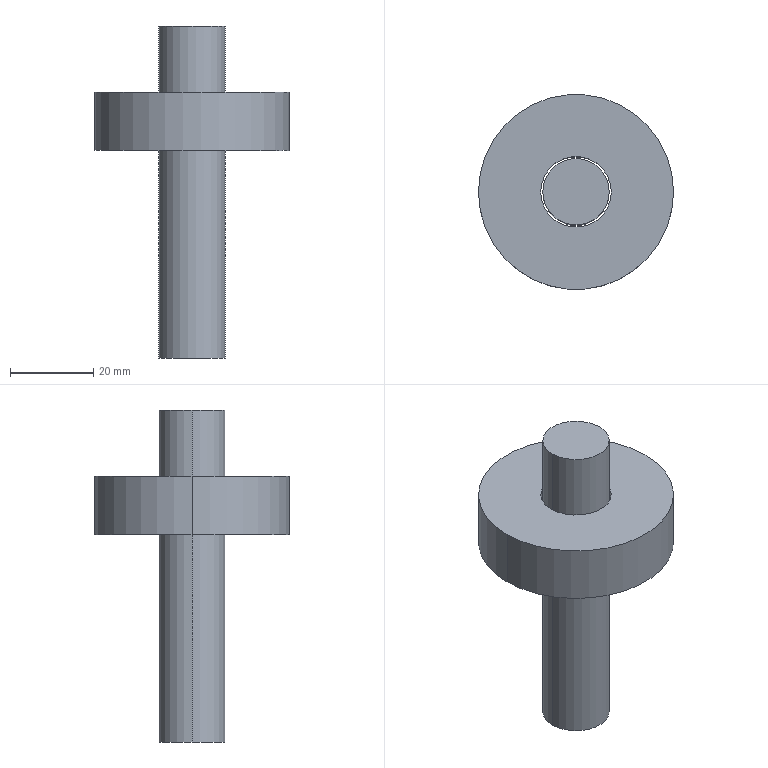Part | STEP file | czesc do docisku llancucha1V11 | 2 solids | 10 faces | box 47 x 47 x 80 mm | volume 37196 mm3 | cylinder 6 | plane 4 | commonest cylinder face diameters 16 x2 17 x2 47 x2
STEP:
#1=CARTESIAN_POINT('',(0.,0.,0.));
#2=DIRECTION('',(0.,0.,1.));
#3=DIRECTION('',(1.,0.,0.));
#4=AXIS2_PLACEMENT_3D('',#1,#2,#3);
#5=CARTESIAN_POINT('',(8.,0.,80.));
#6=VERTEX_POINT('',#5);
#7=CARTESIAN_POINT('',(-8.,0.,80.));
#8=VERTEX_POINT('',#7);
#9=CARTESIAN_POINT('',(0.,0.,80.));
#10=DIRECTION('',(0.,0.,1.));
#11=DIRECTION('',(1.,0.,0.));
#12=AXIS2_PLACEMENT_3D('',#9,#10,#11);
#13=CIRCLE('',#12,8.);
#14=CARTESIAN_POINT('',(0.,0.,80.));
#15=DIRECTION('',(0.,0.,-1.));
#16=DIRECTION('',(-1.,0.,0.));
#17=AXIS2_PLACEMENT_3D('',#14,#15,#16);
#18=CYLINDRICAL_SURFACE('',#17,8.);
#19=CARTESIAN_POINT('',(3.142,0.));
#20=DIRECTION('',(-1.,0.));
#21=VECTOR('',#20,1.);
#22=LINE('',#19,#21);
#23=(GEOMETRIC_REPRESENTATION_CONTEXT(2)PARAMETRIC_REPRESENTATION_CONTEXT()REPRESENTATION_CONTEXT('',''));
#24=DEFINITIONAL_REPRESENTATION('',(#22),#23);
#25=PCURVE('',#18,#24);
#26=CARTESIAN_POINT('',(0.,0.,80.));
#27=DIRECTION('',(0.,0.,1.));
#28=DIRECTION('',(1.,0.,0.));
#29=AXIS2_PLACEMENT_3D('',#26,#27,#28);
#30=PLANE('',#29);
#31=CARTESIAN_POINT('',(0.,0.));
#32=DIRECTION('',(1.,0.));
#33=AXIS2_PLACEMENT_2D('',#31,#32);
#34=CIRCLE('',#33,8.);
#35=(GEOMETRIC_REPRESENTATION_CONTEXT(2)PARAMETRIC_REPRESENTATION_CONTEXT()REPRESENTATION_CONTEXT('',''));
#36=DEFINITIONAL_REPRESENTATION('',(#34),#35);
#37=PCURVE('',#30,#36);
#38=SURFACE_CURVE('',#13,(#25,#37),.PCURVE_S1.);
#39=EDGE_CURVE('',#6,#8,#38,.T.);
#40=ORIENTED_EDGE('',*,*,#39,.F.);
#41=CARTESIAN_POINT('',(8.,0.,0.));
#42=VERTEX_POINT('',#41);
#43=CARTESIAN_POINT('',(8.,0.,80.));
#44=DIRECTION('',(0.,0.,-1.));
#45=VECTOR('',#44,1.);
#46=LINE('',#43,#45);
#47=CARTESIAN_POINT('',(3.142,0.));
#48=DIRECTION('',(0.,1.));
#49=VECTOR('',#48,1.);
#50=LINE('',#47,#49);
#51=(GEOMETRIC_REPRESENTATION_CONTEXT(2)PARAMETRIC_REPRESENTATION_CONTEXT()REPRESENTATION_CONTEXT('',''));
#52=DEFINITIONAL_REPRESENTATION('',(#50),#51);
#53=PCURVE('',#18,#52);
#54=CARTESIAN_POINT('',(0.,0.,80.));
#55=DIRECTION('',(0.,0.,-1.));
#56=DIRECTION('',(-1.,0.,0.));
#57=AXIS2_PLACEMENT_3D('',#54,#55,#56);
#58=CYLINDRICAL_SURFACE('',#57,8.);
#59=CARTESIAN_POINT('',(3.142,0.));
#60=DIRECTION('',(0.,1.));
#61=VECTOR('',#60,1.);
#62=LINE('',#59,#61);
#63=(GEOMETRIC_REPRESENTATION_CONTEXT(2)PARAMETRIC_REPRESENTATION_CONTEXT()REPRESENTATION_CONTEXT('',''));
#64=DEFINITIONAL_REPRESENTATION('',(#62),#63);
#65=PCURVE('',#58,#64);
#66=SURFACE_CURVE('',#46,(#53,#65),.PCURVE_S1.);
#67=EDGE_CURVE('',#6,#42,#66,.T.);
#68=ORIENTED_EDGE('',*,*,#67,.T.);
#69=CARTESIAN_POINT('',(-8.,0.,0.));
#70=VERTEX_POINT('',#69);
#71=CARTESIAN_POINT('',(0.,0.,0.));
#72=DIRECTION('',(0.,0.,1.));
#73=DIRECTION('',(1.,0.,0.));
#74=AXIS2_PLACEMENT_3D('',#71,#72,#73);
#75=CIRCLE('',#74,8.);
#76=CARTESIAN_POINT('',(3.142,80.));
#77=DIRECTION('',(-1.,0.));
#78=VECTOR('',#77,1.);
#79=LINE('',#76,#78);
#80=(GEOMETRIC_REPRESENTATION_CONTEXT(2)PARAMETRIC_REPRESENTATION_CONTEXT()REPRESENTATION_CONTEXT('',''));
#81=DEFINITIONAL_REPRESENTATION('',(#79),#80);
#82=PCURVE('',#18,#81);
#83=CARTESIAN_POINT('',(0.,0.,0.));
#84=DIRECTION('',(0.,0.,1.));
#85=DIRECTION('',(1.,0.,0.));
#86=AXIS2_PLACEMENT_3D('',#83,#84,#85);
#87=PLANE('',#86);
#88=CARTESIAN_POINT('',(0.,0.));
#89=DIRECTION('',(1.,0.));
#90=AXIS2_PLACEMENT_2D('',#88,#89);
#91=CIRCLE('',#90,8.);
#92=(GEOMETRIC_REPRESENTATION_CONTEXT(2)PARAMETRIC_REPRESENTATION_CONTEXT()REPRESENTATION_CONTEXT('',''));
#93=DEFINITIONAL_REPRESENTATION('',(#91),#92);
#94=PCURVE('',#87,#93);
#95=SURFACE_CURVE('',#75,(#82,#94),.PCURVE_S1.);
#96=EDGE_CURVE('',#42,#70,#95,.T.);
#97=ORIENTED_EDGE('',*,*,#96,.T.);
#98=CARTESIAN_POINT('',(-8.,0.,80.));
#99=DIRECTION('',(0.,0.,-1.));
#100=VECTOR('',#99,1.);
#101=LINE('',#98,#100);
#102=CARTESIAN_POINT('',(0.,0.));
#103=DIRECTION('',(0.,1.));
#104=VECTOR('',#103,1.);
#105=LINE('',#102,#104);
#106=(GEOMETRIC_REPRESENTATION_CONTEXT(2)PARAMETRIC_REPRESENTATION_CONTEXT()REPRESENTATION_CONTEXT('',''));
#107=DEFINITIONAL_REPRESENTATION('',(#105),#106);
#108=PCURVE('',#18,#107);
#109=CARTESIAN_POINT('',(6.283,0.));
#110=DIRECTION('',(0.,1.));
#111=VECTOR('',#110,1.);
#112=LINE('',#109,#111);
#113=(GEOMETRIC_REPRESENTATION_CONTEXT(2)PARAMETRIC_REPRESENTATION_CONTEXT()REPRESENTATION_CONTEXT('',''));
#114=DEFINITIONAL_REPRESENTATION('',(#112),#113);
#115=PCURVE('',#58,#114);
#116=SURFACE_CURVE('',#101,(#108,#115),.PCURVE_S1.);
#117=EDGE_CURVE('',#8,#70,#116,.T.);
#118=ORIENTED_EDGE('',*,*,#117,.F.);
#119=EDGE_LOOP('',(#40,#68,#97,#118));
#120=FACE_BOUND('',#119,.T.);
#121=ADVANCED_FACE('',(#120),#18,.T.);
#122=ORIENTED_EDGE('',*,*,#67,.F.);
#123=CARTESIAN_POINT('',(0.,0.,80.));
#124=DIRECTION('',(0.,0.,1.));
#125=DIRECTION('',(1.,0.,0.));
#126=AXIS2_PLACEMENT_3D('',#123,#124,#125);
#127=CIRCLE('',#126,8.);
#128=CARTESIAN_POINT('',(9.425,0.));
#129=DIRECTION('',(-1.,0.));
#130=VECTOR('',#129,1.);
#131=LINE('',#128,#130);
#132=(GEOMETRIC_REPRESENTATION_CONTEXT(2)PARAMETRIC_REPRESENTATION_CONTEXT()REPRESENTATION_CONTEXT('',''));
#133=DEFINITIONAL_REPRESENTATION('',(#131),#132);
#134=PCURVE('',#58,#133);
#135=CARTESIAN_POINT('',(0.,0.));
#136=DIRECTION('',(1.,0.));
#137=AXIS2_PLACEMENT_2D('',#135,#136);
#138=CIRCLE('',#137,8.);
#139=(GEOMETRIC_REPRESENTATION_CONTEXT(2)PARAMETRIC_REPRESENTATION_CONTEXT()REPRESENTATION_CONTEXT('',''));
#140=DEFINITIONAL_REPRESENTATION('',(#138),#139);
#141=PCURVE('',#30,#140);
#142=SURFACE_CURVE('',#127,(#134,#141),.PCURVE_S1.);
#143=EDGE_CURVE('',#8,#6,#142,.T.);
#144=ORIENTED_EDGE('',*,*,#143,.F.);
#145=ORIENTED_EDGE('',*,*,#117,.T.);
#146=CARTESIAN_POINT('',(0.,0.,0.));
#147=DIRECTION('',(0.,0.,1.));
#148=DIRECTION('',(1.,0.,0.));
#149=AXIS2_PLACEMENT_3D('',#146,#147,#148);
#150=CIRCLE('',#149,8.);
#151=CARTESIAN_POINT('',(9.425,80.));
#152=DIRECTION('',(-1.,0.));
#153=VECTOR('',#152,1.);
#154=LINE('',#151,#153);
#155=(GEOMETRIC_REPRESENTATION_CONTEXT(2)PARAMETRIC_REPRESENTATION_CONTEXT()REPRESENTATION_CONTEXT('',''));
#156=DEFINITIONAL_REPRESENTATION('',(#154),#155);
#157=PCURVE('',#58,#156);
#158=CARTESIAN_POINT('',(0.,0.));
#159=DIRECTION('',(1.,0.));
#160=AXIS2_PLACEMENT_2D('',#158,#159);
#161=CIRCLE('',#160,8.);
#162=(GEOMETRIC_REPRESENTATION_CONTEXT(2)PARAMETRIC_REPRESENTATION_CONTEXT()REPRESENTATION_CONTEXT('',''));
#163=DEFINITIONAL_REPRESENTATION('',(#161),#162);
#164=PCURVE('',#87,#163);
#165=SURFACE_CURVE('',#150,(#157,#164),.PCURVE_S1.);
#166=EDGE_CURVE('',#70,#42,#165,.T.);
#167=ORIENTED_EDGE('',*,*,#166,.T.);
#168=EDGE_LOOP('',(#122,#144,#145,#167));
#169=FACE_BOUND('',#168,.T.);
#170=ADVANCED_FACE('',(#169),#58,.T.);
#171=ORIENTED_EDGE('',*,*,#143,.T.);
#172=ORIENTED_EDGE('',*,*,#39,.T.);
#173=EDGE_LOOP('',(#171,#172));
#174=FACE_BOUND('',#173,.T.);
#175=ADVANCED_FACE('',(#174),#30,.T.);
#176=ORIENTED_EDGE('',*,*,#166,.F.);
#177=ORIENTED_EDGE('',*,*,#96,.F.);
#178=EDGE_LOOP('',(#176,#177));
#179=FACE_BOUND('',#178,.T.);
#180=ADVANCED_FACE('',(#179),#87,.F.);
#181=CLOSED_SHELL('',(#121,#170,#175,#180));
#182=MANIFOLD_SOLID_BREP('',#181);
#183=CARTESIAN_POINT('',(-8.5,0.,64.));
#184=VERTEX_POINT('',#183);
#185=CARTESIAN_POINT('',(-8.5,0.,50.));
#186=VERTEX_POINT('',#185);
#187=CARTESIAN_POINT('',(-8.5,0.,64.));
#188=DIRECTION('',(0.,0.,-1.));
#189=VECTOR('',#188,1.);
#190=LINE('',#187,#189);
#191=CARTESIAN_POINT('',(0.,0.,64.));
#192=DIRECTION('',(0.,0.,-1.));
#193=DIRECTION('',(-1.,0.,0.));
#194=AXIS2_PLACEMENT_3D('',#191,#192,#193);
#195=CYLINDRICAL_SURFACE('',#194,8.5);
#196=CARTESIAN_POINT('',(6.283,0.));
#197=DIRECTION('',(0.,1.));
#198=VECTOR('',#197,1.);
#199=LINE('',#196,#198);
#200=(GEOMETRIC_REPRESENTATION_CONTEXT(2)PARAMETRIC_REPRESENTATION_CONTEXT()REPRESENTATION_CONTEXT('',''));
#201=DEFINITIONAL_REPRESENTATION('',(#199),#200);
#202=PCURVE('',#195,#201);
#203=CARTESIAN_POINT('',(0.,0.,64.));
#204=DIRECTION('',(0.,0.,-1.));
#205=DIRECTION('',(-1.,0.,0.));
#206=AXIS2_PLACEMENT_3D('',#203,#204,#205);
#207=CYLINDRICAL_SURFACE('',#206,8.5);
#208=CARTESIAN_POINT('',(0.,0.));
#209=DIRECTION('',(0.,1.));
#210=VECTOR('',#209,1.);
#211=LINE('',#208,#210);
#212=(GEOMETRIC_REPRESENTATION_CONTEXT(2)PARAMETRIC_REPRESENTATION_CONTEXT()REPRESENTATION_CONTEXT('',''));
#213=DEFINITIONAL_REPRESENTATION('',(#211),#212);
#214=PCURVE('',#207,#213);
#215=SURFACE_CURVE('',#190,(#202,#214),.PCURVE_S1.);
#216=EDGE_CURVE('',#184,#186,#215,.T.);
#217=ORIENTED_EDGE('',*,*,#216,.T.);
#218=CARTESIAN_POINT('',(8.5,0.,50.));
#219=VERTEX_POINT('',#218);
#220=CARTESIAN_POINT('',(0.,0.,50.));
#221=DIRECTION('',(0.,0.,1.));
#222=DIRECTION('',(1.,0.,0.));
#223=AXIS2_PLACEMENT_3D('',#220,#221,#222);
#224=CIRCLE('',#223,8.5);
#225=CARTESIAN_POINT('',(9.425,14.));
#226=DIRECTION('',(-1.,0.));
#227=VECTOR('',#226,1.);
#228=LINE('',#225,#227);
#229=(GEOMETRIC_REPRESENTATION_CONTEXT(2)PARAMETRIC_REPRESENTATION_CONTEXT()REPRESENTATION_CONTEXT('',''));
#230=DEFINITIONAL_REPRESENTATION('',(#228),#229);
#231=PCURVE('',#195,#230);
#232=CARTESIAN_POINT('',(0.,0.,50.));
#233=DIRECTION('',(0.,0.,1.));
#234=DIRECTION('',(1.,0.,0.));
#235=AXIS2_PLACEMENT_3D('',#232,#233,#234);
#236=PLANE('',#235);
#237=CARTESIAN_POINT('',(0.,0.));
#238=DIRECTION('',(1.,0.));
#239=AXIS2_PLACEMENT_2D('',#237,#238);
#240=CIRCLE('',#239,8.5);
#241=(GEOMETRIC_REPRESENTATION_CONTEXT(2)PARAMETRIC_REPRESENTATION_CONTEXT()REPRESENTATION_CONTEXT('',''));
#242=DEFINITIONAL_REPRESENTATION('',(#240),#241);
#243=PCURVE('',#236,#242);
#244=SURFACE_CURVE('',#224,(#231,#243),.PCURVE_S1.);
#245=EDGE_CURVE('',#186,#219,#244,.T.);
#246=ORIENTED_EDGE('',*,*,#245,.T.);
#247=CARTESIAN_POINT('',(8.5,0.,64.));
#248=VERTEX_POINT('',#247);
#249=CARTESIAN_POINT('',(8.5,0.,64.));
#250=DIRECTION('',(0.,0.,-1.));
#251=VECTOR('',#250,1.);
#252=LINE('',#249,#251);
#253=CARTESIAN_POINT('',(3.142,0.));
#254=DIRECTION('',(0.,1.));
#255=VECTOR('',#254,1.);
#256=LINE('',#253,#255);
#257=(GEOMETRIC_REPRESENTATION_CONTEXT(2)PARAMETRIC_REPRESENTATION_CONTEXT()REPRESENTATION_CONTEXT('',''));
#258=DEFINITIONAL_REPRESENTATION('',(#256),#257);
#259=PCURVE('',#195,#258);
#260=CARTESIAN_POINT('',(3.142,0.));
#261=DIRECTION('',(0.,1.));
#262=VECTOR('',#261,1.);
#263=LINE('',#260,#262);
#264=(GEOMETRIC_REPRESENTATION_CONTEXT(2)PARAMETRIC_REPRESENTATION_CONTEXT()REPRESENTATION_CONTEXT('',''));
#265=DEFINITIONAL_REPRESENTATION('',(#263),#264);
#266=PCURVE('',#207,#265);
#267=SURFACE_CURVE('',#252,(#259,#266),.PCURVE_S1.);
#268=EDGE_CURVE('',#248,#219,#267,.T.);
#269=ORIENTED_EDGE('',*,*,#268,.F.);
#270=CARTESIAN_POINT('',(0.,0.,64.));
#271=DIRECTION('',(0.,0.,1.));
#272=DIRECTION('',(1.,0.,0.));
#273=AXIS2_PLACEMENT_3D('',#270,#271,#272);
#274=CIRCLE('',#273,8.5);
#275=CARTESIAN_POINT('',(9.425,0.));
#276=DIRECTION('',(-1.,0.));
#277=VECTOR('',#276,1.);
#278=LINE('',#275,#277);
#279=(GEOMETRIC_REPRESENTATION_CONTEXT(2)PARAMETRIC_REPRESENTATION_CONTEXT()REPRESENTATION_CONTEXT('',''));
#280=DEFINITIONAL_REPRESENTATION('',(#278),#279);
#281=PCURVE('',#195,#280);
#282=CARTESIAN_POINT('',(0.,0.,64.));
#283=DIRECTION('',(0.,0.,1.));
#284=DIRECTION('',(1.,0.,0.));
#285=AXIS2_PLACEMENT_3D('',#282,#283,#284);
#286=PLANE('',#285);
#287=CARTESIAN_POINT('',(0.,0.));
#288=DIRECTION('',(1.,0.));
#289=AXIS2_PLACEMENT_2D('',#287,#288);
#290=CIRCLE('',#289,8.5);
#291=(GEOMETRIC_REPRESENTATION_CONTEXT(2)PARAMETRIC_REPRESENTATION_CONTEXT()REPRESENTATION_CONTEXT('',''));
#292=DEFINITIONAL_REPRESENTATION('',(#290),#291);
#293=PCURVE('',#286,#292);
#294=SURFACE_CURVE('',#274,(#281,#293),.PCURVE_S1.);
#295=EDGE_CURVE('',#184,#248,#294,.T.);
#296=ORIENTED_EDGE('',*,*,#295,.F.);
#297=EDGE_LOOP('',(#217,#246,#269,#296));
#298=FACE_BOUND('',#297,.F.);
#299=ADVANCED_FACE('',(#298),#195,.F.);
#300=CARTESIAN_POINT('',(23.5,0.,64.));
#301=VERTEX_POINT('',#300);
#302=CARTESIAN_POINT('',(-23.5,0.,64.));
#303=VERTEX_POINT('',#302);
#304=CARTESIAN_POINT('',(0.,0.,64.));
#305=DIRECTION('',(0.,0.,1.));
#306=DIRECTION('',(1.,0.,0.));
#307=AXIS2_PLACEMENT_3D('',#304,#305,#306);
#308=CIRCLE('',#307,23.5);
#309=CARTESIAN_POINT('',(0.,0.,64.));
#310=DIRECTION('',(0.,0.,-1.));
#311=DIRECTION('',(-1.,0.,0.));
#312=AXIS2_PLACEMENT_3D('',#309,#310,#311);
#313=CYLINDRICAL_SURFACE('',#312,23.5);
#314=CARTESIAN_POINT('',(3.142,0.));
#315=DIRECTION('',(-1.,0.));
#316=VECTOR('',#315,1.);
#317=LINE('',#314,#316);
#318=(GEOMETRIC_REPRESENTATION_CONTEXT(2)PARAMETRIC_REPRESENTATION_CONTEXT()REPRESENTATION_CONTEXT('',''));
#319=DEFINITIONAL_REPRESENTATION('',(#317),#318);
#320=PCURVE('',#313,#319);
#321=CARTESIAN_POINT('',(0.,0.));
#322=DIRECTION('',(1.,0.));
#323=AXIS2_PLACEMENT_2D('',#321,#322);
#324=CIRCLE('',#323,23.5);
#325=(GEOMETRIC_REPRESENTATION_CONTEXT(2)PARAMETRIC_REPRESENTATION_CONTEXT()REPRESENTATION_CONTEXT('',''));
#326=DEFINITIONAL_REPRESENTATION('',(#324),#325);
#327=PCURVE('',#286,#326);
#328=SURFACE_CURVE('',#308,(#320,#327),.PCURVE_S1.);
#329=EDGE_CURVE('',#301,#303,#328,.T.);
#330=ORIENTED_EDGE('',*,*,#329,.F.);
#331=CARTESIAN_POINT('',(23.5,0.,50.));
#332=VERTEX_POINT('',#331);
#333=CARTESIAN_POINT('',(23.5,0.,64.));
#334=DIRECTION('',(0.,0.,-1.));
#335=VECTOR('',#334,1.);
#336=LINE('',#333,#335);
#337=CARTESIAN_POINT('',(3.142,0.));
#338=DIRECTION('',(0.,1.));
#339=VECTOR('',#338,1.);
#340=LINE('',#337,#339);
#341=(GEOMETRIC_REPRESENTATION_CONTEXT(2)PARAMETRIC_REPRESENTATION_CONTEXT()REPRESENTATION_CONTEXT('',''));
#342=DEFINITIONAL_REPRESENTATION('',(#340),#341);
#343=PCURVE('',#313,#342);
#344=CARTESIAN_POINT('',(0.,0.,64.));
#345=DIRECTION('',(0.,0.,-1.));
#346=DIRECTION('',(-1.,0.,0.));
#347=AXIS2_PLACEMENT_3D('',#344,#345,#346);
#348=CYLINDRICAL_SURFACE('',#347,23.5);
#349=CARTESIAN_POINT('',(3.142,0.));
#350=DIRECTION('',(0.,1.));
#351=VECTOR('',#350,1.);
#352=LINE('',#349,#351);
#353=(GEOMETRIC_REPRESENTATION_CONTEXT(2)PARAMETRIC_REPRESENTATION_CONTEXT()REPRESENTATION_CONTEXT('',''));
#354=DEFINITIONAL_REPRESENTATION('',(#352),#353);
#355=PCURVE('',#348,#354);
#356=SURFACE_CURVE('',#336,(#343,#355),.PCURVE_S1.);
#357=EDGE_CURVE('',#301,#332,#356,.T.);
#358=ORIENTED_EDGE('',*,*,#357,.T.);
#359=CARTESIAN_POINT('',(-23.5,0.,50.));
#360=VERTEX_POINT('',#359);
#361=CARTESIAN_POINT('',(0.,0.,50.));
#362=DIRECTION('',(0.,0.,1.));
#363=DIRECTION('',(1.,0.,0.));
#364=AXIS2_PLACEMENT_3D('',#361,#362,#363);
#365=CIRCLE('',#364,23.5);
#366=CARTESIAN_POINT('',(3.142,14.));
#367=DIRECTION('',(-1.,0.));
#368=VECTOR('',#367,1.);
#369=LINE('',#366,#368);
#370=(GEOMETRIC_REPRESENTATION_CONTEXT(2)PARAMETRIC_REPRESENTATION_CONTEXT()REPRESENTATION_CONTEXT('',''));
#371=DEFINITIONAL_REPRESENTATION('',(#369),#370);
#372=PCURVE('',#313,#371);
#373=CARTESIAN_POINT('',(0.,0.));
#374=DIRECTION('',(1.,0.));
#375=AXIS2_PLACEMENT_2D('',#373,#374);
#376=CIRCLE('',#375,23.5);
#377=(GEOMETRIC_REPRESENTATION_CONTEXT(2)PARAMETRIC_REPRESENTATION_CONTEXT()REPRESENTATION_CONTEXT('',''));
#378=DEFINITIONAL_REPRESENTATION('',(#376),#377);
#379=PCURVE('',#236,#378);
#380=SURFACE_CURVE('',#365,(#372,#379),.PCURVE_S1.);
#381=EDGE_CURVE('',#332,#360,#380,.T.);
#382=ORIENTED_EDGE('',*,*,#381,.T.);
#383=CARTESIAN_POINT('',(-23.5,0.,64.));
#384=DIRECTION('',(0.,0.,-1.));
#385=VECTOR('',#384,1.);
#386=LINE('',#383,#385);
#387=CARTESIAN_POINT('',(0.,0.));
#388=DIRECTION('',(0.,1.));
#389=VECTOR('',#388,1.);
#390=LINE('',#387,#389);
#391=(GEOMETRIC_REPRESENTATION_CONTEXT(2)PARAMETRIC_REPRESENTATION_CONTEXT()REPRESENTATION_CONTEXT('',''));
#392=DEFINITIONAL_REPRESENTATION('',(#390),#391);
#393=PCURVE('',#313,#392);
#394=CARTESIAN_POINT('',(6.283,0.));
#395=DIRECTION('',(0.,1.));
#396=VECTOR('',#395,1.);
#397=LINE('',#394,#396);
#398=(GEOMETRIC_REPRESENTATION_CONTEXT(2)PARAMETRIC_REPRESENTATION_CONTEXT()REPRESENTATION_CONTEXT('',''));
#399=DEFINITIONAL_REPRESENTATION('',(#397),#398);
#400=PCURVE('',#348,#399);
#401=SURFACE_CURVE('',#386,(#393,#400),.PCURVE_S1.);
#402=EDGE_CURVE('',#303,#360,#401,.T.);
#403=ORIENTED_EDGE('',*,*,#402,.F.);
#404=EDGE_LOOP('',(#330,#358,#382,#403));
#405=FACE_BOUND('',#404,.T.);
#406=ADVANCED_FACE('',(#405),#313,.T.);
#407=CARTESIAN_POINT('',(0.,0.,64.));
#408=DIRECTION('',(0.,0.,1.));
#409=DIRECTION('',(1.,0.,0.));
#410=AXIS2_PLACEMENT_3D('',#407,#408,#409);
#411=CIRCLE('',#410,23.5);
#412=CARTESIAN_POINT('',(0.,0.));
#413=DIRECTION('',(1.,0.));
#414=AXIS2_PLACEMENT_2D('',#412,#413);
#415=CIRCLE('',#414,23.5);
#416=(GEOMETRIC_REPRESENTATION_CONTEXT(2)PARAMETRIC_REPRESENTATION_CONTEXT()REPRESENTATION_CONTEXT('',''));
#417=DEFINITIONAL_REPRESENTATION('',(#415),#416);
#418=PCURVE('',#286,#417);
#419=CARTESIAN_POINT('',(9.425,0.));
#420=DIRECTION('',(-1.,0.));
#421=VECTOR('',#420,1.);
#422=LINE('',#419,#421);
#423=(GEOMETRIC_REPRESENTATION_CONTEXT(2)PARAMETRIC_REPRESENTATION_CONTEXT()REPRESENTATION_CONTEXT('',''));
#424=DEFINITIONAL_REPRESENTATION('',(#422),#423);
#425=PCURVE('',#348,#424);
#426=SURFACE_CURVE('',#411,(#418,#425),.PCURVE_S1.);
#427=EDGE_CURVE('',#303,#301,#426,.T.);
#428=ORIENTED_EDGE('',*,*,#427,.T.);
#429=ORIENTED_EDGE('',*,*,#329,.T.);
#430=EDGE_LOOP('',(#428,#429));
#431=FACE_BOUND('',#430,.T.);
#432=ORIENTED_EDGE('',*,*,#295,.F.);
#433=CARTESIAN_POINT('',(0.,0.,64.));
#434=DIRECTION('',(0.,0.,1.));
#435=DIRECTION('',(1.,0.,0.));
#436=AXIS2_PLACEMENT_3D('',#433,#434,#435);
#437=CIRCLE('',#436,8.5);
#438=CARTESIAN_POINT('',(0.,0.));
#439=DIRECTION('',(1.,0.));
#440=AXIS2_PLACEMENT_2D('',#438,#439);
#441=CIRCLE('',#440,8.5);
#442=(GEOMETRIC_REPRESENTATION_CONTEXT(2)PARAMETRIC_REPRESENTATION_CONTEXT()REPRESENTATION_CONTEXT('',''));
#443=DEFINITIONAL_REPRESENTATION('',(#441),#442);
#444=PCURVE('',#286,#443);
#445=CARTESIAN_POINT('',(3.142,0.));
#446=DIRECTION('',(-1.,0.));
#447=VECTOR('',#446,1.);
#448=LINE('',#445,#447);
#449=(GEOMETRIC_REPRESENTATION_CONTEXT(2)PARAMETRIC_REPRESENTATION_CONTEXT()REPRESENTATION_CONTEXT('',''));
#450=DEFINITIONAL_REPRESENTATION('',(#448),#449);
#451=PCURVE('',#207,#450);
#452=SURFACE_CURVE('',#437,(#444,#451),.PCURVE_S1.);
#453=EDGE_CURVE('',#248,#184,#452,.T.);
#454=ORIENTED_EDGE('',*,*,#453,.F.);
#455=EDGE_LOOP('',(#432,#454));
#456=FACE_BOUND('',#455,.T.);
#457=ADVANCED_FACE('',(#431,#456),#286,.T.);
#458=CARTESIAN_POINT('',(0.,0.,50.));
#459=DIRECTION('',(0.,0.,1.));
#460=DIRECTION('',(1.,0.,0.));
#461=AXIS2_PLACEMENT_3D('',#458,#459,#460);
#462=CIRCLE('',#461,23.5);
#463=CARTESIAN_POINT('',(0.,0.));
#464=DIRECTION('',(1.,0.));
#465=AXIS2_PLACEMENT_2D('',#463,#464);
#466=CIRCLE('',#465,23.5);
#467=(GEOMETRIC_REPRESENTATION_CONTEXT(2)PARAMETRIC_REPRESENTATION_CONTEXT()REPRESENTATION_CONTEXT('',''));
#468=DEFINITIONAL_REPRESENTATION('',(#466),#467);
#469=PCURVE('',#236,#468);
#470=CARTESIAN_POINT('',(9.425,14.));
#471=DIRECTION('',(-1.,0.));
#472=VECTOR('',#471,1.);
#473=LINE('',#470,#472);
#474=(GEOMETRIC_REPRESENTATION_CONTEXT(2)PARAMETRIC_REPRESENTATION_CONTEXT()REPRESENTATION_CONTEXT('',''));
#475=DEFINITIONAL_REPRESENTATION('',(#473),#474);
#476=PCURVE('',#348,#475);
#477=SURFACE_CURVE('',#462,(#469,#476),.PCURVE_S1.);
#478=EDGE_CURVE('',#360,#332,#477,.T.);
#479=ORIENTED_EDGE('',*,*,#478,.F.);
#480=ORIENTED_EDGE('',*,*,#381,.F.);
#481=EDGE_LOOP('',(#479,#480));
#482=FACE_BOUND('',#481,.T.);
#483=ORIENTED_EDGE('',*,*,#245,.T.);
#484=CARTESIAN_POINT('',(0.,0.,50.));
#485=DIRECTION('',(0.,0.,1.));
#486=DIRECTION('',(1.,0.,0.));
#487=AXIS2_PLACEMENT_3D('',#484,#485,#486);
#488=CIRCLE('',#487,8.5);
#489=CARTESIAN_POINT('',(0.,0.));
#490=DIRECTION('',(1.,0.));
#491=AXIS2_PLACEMENT_2D('',#489,#490);
#492=CIRCLE('',#491,8.5);
#493=(GEOMETRIC_REPRESENTATION_CONTEXT(2)PARAMETRIC_REPRESENTATION_CONTEXT()REPRESENTATION_CONTEXT('',''));
#494=DEFINITIONAL_REPRESENTATION('',(#492),#493);
#495=PCURVE('',#236,#494);
#496=CARTESIAN_POINT('',(3.142,14.));
#497=DIRECTION('',(-1.,0.));
#498=VECTOR('',#497,1.);
#499=LINE('',#496,#498);
#500=(GEOMETRIC_REPRESENTATION_CONTEXT(2)PARAMETRIC_REPRESENTATION_CONTEXT()REPRESENTATION_CONTEXT('',''));
#501=DEFINITIONAL_REPRESENTATION('',(#499),#500);
#502=PCURVE('',#207,#501);
#503=SURFACE_CURVE('',#488,(#495,#502),.PCURVE_S1.);
#504=EDGE_CURVE('',#219,#186,#503,.T.);
#505=ORIENTED_EDGE('',*,*,#504,.T.);
#506=EDGE_LOOP('',(#483,#505));
#507=FACE_BOUND('',#506,.T.);
#508=ADVANCED_FACE('',(#482,#507),#236,.F.);
#509=ORIENTED_EDGE('',*,*,#357,.F.);
#510=ORIENTED_EDGE('',*,*,#427,.F.);
#511=ORIENTED_EDGE('',*,*,#402,.T.);
#512=ORIENTED_EDGE('',*,*,#478,.T.);
#513=EDGE_LOOP('',(#509,#510,#511,#512));
#514=FACE_BOUND('',#513,.T.);
#515=ADVANCED_FACE('',(#514),#348,.T.);
#516=ORIENTED_EDGE('',*,*,#504,.T.);
#517=ORIENTED_EDGE('',*,*,#216,.F.);
#518=ORIENTED_EDGE('',*,*,#453,.F.);
#519=ORIENTED_EDGE('',*,*,#268,.T.);
#520=EDGE_LOOP('',(#516,#517,#518,#519));
#521=FACE_BOUND('',#520,.F.);
#522=ADVANCED_FACE('',(#521),#207,.F.);
#523=CLOSED_SHELL('',(#299,#406,#457,#508,#515,#522));
#524=MANIFOLD_SOLID_BREP('',#523);
#525=(LENGTH_UNIT()NAMED_UNIT(*)SI_UNIT(.MILLI.,.METRE.));
#526=UNCERTAINTY_MEASURE_WITH_UNIT(LENGTH_MEASURE(0.0000001),#525,'','');
#527=(NAMED_UNIT(*)PLANE_ANGLE_UNIT()SI_UNIT($,.RADIAN.));
#528=(NAMED_UNIT(*)SI_UNIT($,.STERADIAN.)SOLID_ANGLE_UNIT());
#529=(GEOMETRIC_REPRESENTATION_CONTEXT(3)GLOBAL_UNCERTAINTY_ASSIGNED_CONTEXT((#526))GLOBAL_UNIT_ASSIGNED_CONTEXT((#525,#527,#528))REPRESENTATION_CONTEXT('',''));
#530=SHAPE_REPRESENTATION('',(#4,#182,#524),#529);